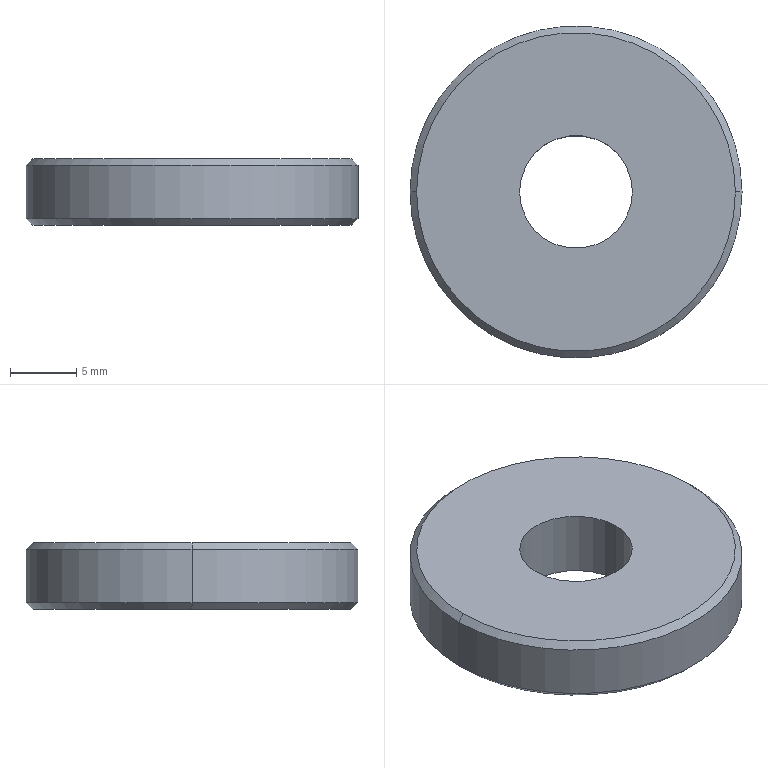Part | STEP file | PN_0013 Press plate | 1 solid | 10 faces | box 25 x 25 x 5 mm | volume 2151 mm3 | cylinder 4 | cone 4 | plane 2 | commonest cylinder face diameters 8.5 x2 25 x2
STEP:
#1=CARTESIAN_POINT('',(0.,0.,0.));
#2=DIRECTION('',(0.,0.,1.));
#3=DIRECTION('',(1.,0.,0.));
#4=AXIS2_PLACEMENT_3D('',#1,#2,#3);
#5=CARTESIAN_POINT('',(-4.25,0.,5.));
#6=VERTEX_POINT('',#5);
#7=CARTESIAN_POINT('',(-4.25,0.,0.));
#8=VERTEX_POINT('',#7);
#9=CARTESIAN_POINT('',(-4.25,0.,5.));
#10=DIRECTION('',(0.,0.,-1.));
#11=VECTOR('',#10,1.);
#12=LINE('',#9,#11);
#13=CARTESIAN_POINT('',(0.,0.,5.));
#14=DIRECTION('',(0.,0.,-1.));
#15=DIRECTION('',(-1.,0.,0.));
#16=AXIS2_PLACEMENT_3D('',#13,#14,#15);
#17=CYLINDRICAL_SURFACE('',#16,4.25);
#18=CARTESIAN_POINT('',(6.283,0.));
#19=DIRECTION('',(0.,1.));
#20=VECTOR('',#19,1.);
#21=LINE('',#18,#20);
#22=(GEOMETRIC_REPRESENTATION_CONTEXT(2)PARAMETRIC_REPRESENTATION_CONTEXT()REPRESENTATION_CONTEXT('',''));
#23=DEFINITIONAL_REPRESENTATION('',(#21),#22);
#24=PCURVE('',#17,#23);
#25=CARTESIAN_POINT('',(0.,0.,5.));
#26=DIRECTION('',(0.,0.,-1.));
#27=DIRECTION('',(-1.,0.,0.));
#28=AXIS2_PLACEMENT_3D('',#25,#26,#27);
#29=CYLINDRICAL_SURFACE('',#28,4.25);
#30=CARTESIAN_POINT('',(0.,0.));
#31=DIRECTION('',(0.,1.));
#32=VECTOR('',#31,1.);
#33=LINE('',#30,#32);
#34=(GEOMETRIC_REPRESENTATION_CONTEXT(2)PARAMETRIC_REPRESENTATION_CONTEXT()REPRESENTATION_CONTEXT('',''));
#35=DEFINITIONAL_REPRESENTATION('',(#33),#34);
#36=PCURVE('',#29,#35);
#37=SURFACE_CURVE('',#12,(#24,#36),.PCURVE_S1.);
#38=EDGE_CURVE('',#6,#8,#37,.T.);
#39=ORIENTED_EDGE('',*,*,#38,.T.);
#40=CARTESIAN_POINT('',(4.25,0.,0.));
#41=VERTEX_POINT('',#40);
#42=CARTESIAN_POINT('',(0.,0.,0.));
#43=DIRECTION('',(0.,0.,-1.));
#44=DIRECTION('',(-1.,0.,0.));
#45=AXIS2_PLACEMENT_3D('',#42,#43,#44);
#46=CIRCLE('',#45,4.25);
#47=CARTESIAN_POINT('',(0.,5.));
#48=DIRECTION('',(1.,0.));
#49=VECTOR('',#48,1.);
#50=LINE('',#47,#49);
#51=(GEOMETRIC_REPRESENTATION_CONTEXT(2)PARAMETRIC_REPRESENTATION_CONTEXT()REPRESENTATION_CONTEXT('',''));
#52=DEFINITIONAL_REPRESENTATION('',(#50),#51);
#53=PCURVE('',#17,#52);
#54=CARTESIAN_POINT('',(0.,0.,0.));
#55=DIRECTION('',(0.,0.,1.));
#56=DIRECTION('',(1.,0.,0.));
#57=AXIS2_PLACEMENT_3D('',#54,#55,#56);
#58=PLANE('',#57);
#59=CARTESIAN_POINT('',(-4.25,0.));
#60=CARTESIAN_POINT('',(-4.25,7.361));
#61=CARTESIAN_POINT('',(2.125,3.681));
#62=CARTESIAN_POINT('',(8.5,0.));
#63=CARTESIAN_POINT('',(2.125,-3.681));
#64=CARTESIAN_POINT('',(-4.25,-7.361));
#65=CARTESIAN_POINT('',(-4.25,0.));
#66=(BOUNDED_CURVE()B_SPLINE_CURVE(2,(#59,#60,#61,#62,#63,#64,#65),.UNSPECIFIED.,.T.,.F.)B_SPLINE_CURVE_WITH_KNOTS((1,2,2,2,2,1),(-2.094,0.,2.094,4.189,6.283,8.378),.UNSPECIFIED.)CURVE()GEOMETRIC_REPRESENTATION_ITEM()RATIONAL_B_SPLINE_CURVE((1.,0.5,1.,0.5,1.,0.5,1.))REPRESENTATION_ITEM(''));
#67=(GEOMETRIC_REPRESENTATION_CONTEXT(2)PARAMETRIC_REPRESENTATION_CONTEXT()REPRESENTATION_CONTEXT('',''));
#68=DEFINITIONAL_REPRESENTATION('',(#66),#67);
#69=PCURVE('',#58,#68);
#70=SURFACE_CURVE('',#46,(#53,#69),.PCURVE_S1.);
#71=EDGE_CURVE('',#41,#8,#70,.T.);
#72=ORIENTED_EDGE('',*,*,#71,.F.);
#73=CARTESIAN_POINT('',(4.25,0.,5.));
#74=VERTEX_POINT('',#73);
#75=CARTESIAN_POINT('',(4.25,0.,5.));
#76=DIRECTION('',(0.,0.,-1.));
#77=VECTOR('',#76,1.);
#78=LINE('',#75,#77);
#79=CARTESIAN_POINT('',(3.142,0.));
#80=DIRECTION('',(0.,1.));
#81=VECTOR('',#80,1.);
#82=LINE('',#79,#81);
#83=(GEOMETRIC_REPRESENTATION_CONTEXT(2)PARAMETRIC_REPRESENTATION_CONTEXT()REPRESENTATION_CONTEXT('',''));
#84=DEFINITIONAL_REPRESENTATION('',(#82),#83);
#85=PCURVE('',#17,#84);
#86=CARTESIAN_POINT('',(3.142,0.));
#87=DIRECTION('',(0.,1.));
#88=VECTOR('',#87,1.);
#89=LINE('',#86,#88);
#90=(GEOMETRIC_REPRESENTATION_CONTEXT(2)PARAMETRIC_REPRESENTATION_CONTEXT()REPRESENTATION_CONTEXT('',''));
#91=DEFINITIONAL_REPRESENTATION('',(#89),#90);
#92=PCURVE('',#29,#91);
#93=SURFACE_CURVE('',#78,(#85,#92),.PCURVE_S1.);
#94=EDGE_CURVE('',#74,#41,#93,.T.);
#95=ORIENTED_EDGE('',*,*,#94,.F.);
#96=CARTESIAN_POINT('',(0.,0.,5.));
#97=DIRECTION('',(0.,0.,-1.));
#98=DIRECTION('',(-1.,0.,0.));
#99=AXIS2_PLACEMENT_3D('',#96,#97,#98);
#100=CIRCLE('',#99,4.25);
#101=CARTESIAN_POINT('',(0.,0.));
#102=DIRECTION('',(1.,0.));
#103=VECTOR('',#102,1.);
#104=LINE('',#101,#103);
#105=(GEOMETRIC_REPRESENTATION_CONTEXT(2)PARAMETRIC_REPRESENTATION_CONTEXT()REPRESENTATION_CONTEXT('',''));
#106=DEFINITIONAL_REPRESENTATION('',(#104),#105);
#107=PCURVE('',#17,#106);
#108=CARTESIAN_POINT('',(0.,0.,5.));
#109=DIRECTION('',(0.,0.,1.));
#110=DIRECTION('',(1.,0.,0.));
#111=AXIS2_PLACEMENT_3D('',#108,#109,#110);
#112=PLANE('',#111);
#113=CARTESIAN_POINT('',(-4.25,0.));
#114=CARTESIAN_POINT('',(-4.25,7.361));
#115=CARTESIAN_POINT('',(2.125,3.681));
#116=CARTESIAN_POINT('',(8.5,0.));
#117=CARTESIAN_POINT('',(2.125,-3.681));
#118=CARTESIAN_POINT('',(-4.25,-7.361));
#119=CARTESIAN_POINT('',(-4.25,0.));
#120=(BOUNDED_CURVE()B_SPLINE_CURVE(2,(#113,#114,#115,#116,#117,#118,#119),.UNSPECIFIED.,.T.,.F.)B_SPLINE_CURVE_WITH_KNOTS((1,2,2,2,2,1),(-2.094,0.,2.094,4.189,6.283,8.378),.UNSPECIFIED.)CURVE()GEOMETRIC_REPRESENTATION_ITEM()RATIONAL_B_SPLINE_CURVE((1.,0.5,1.,0.5,1.,0.5,1.))REPRESENTATION_ITEM(''));
#121=(GEOMETRIC_REPRESENTATION_CONTEXT(2)PARAMETRIC_REPRESENTATION_CONTEXT()REPRESENTATION_CONTEXT('',''));
#122=DEFINITIONAL_REPRESENTATION('',(#120),#121);
#123=PCURVE('',#112,#122);
#124=SURFACE_CURVE('',#100,(#107,#123),.PCURVE_S1.);
#125=EDGE_CURVE('',#74,#6,#124,.T.);
#126=ORIENTED_EDGE('',*,*,#125,.T.);
#127=EDGE_LOOP('',(#39,#72,#95,#126));
#128=FACE_BOUND('',#127,.F.);
#129=ADVANCED_FACE('',(#128),#17,.F.);
#130=CARTESIAN_POINT('',(12.,0.,0.));
#131=VERTEX_POINT('',#130);
#132=CARTESIAN_POINT('',(-12.,0.,0.));
#133=VERTEX_POINT('',#132);
#134=CARTESIAN_POINT('',(0.,0.,0.));
#135=DIRECTION('',(0.,0.,1.));
#136=DIRECTION('',(1.,0.,0.));
#137=AXIS2_PLACEMENT_3D('',#134,#135,#136);
#138=CIRCLE('',#137,12.);
#139=CARTESIAN_POINT('',(0.,0.,0.5));
#140=DIRECTION('',(0.,0.,1.));
#141=DIRECTION('',(1.,0.,0.));
#142=AXIS2_PLACEMENT_3D('',#139,#140,#141);
#143=CONICAL_SURFACE('',#142,12.5,0.7854);
#144=CARTESIAN_POINT('',(0.,-0.5));
#145=DIRECTION('',(1.,0.));
#146=VECTOR('',#145,1.);
#147=LINE('',#144,#146);
#148=(GEOMETRIC_REPRESENTATION_CONTEXT(2)PARAMETRIC_REPRESENTATION_CONTEXT()REPRESENTATION_CONTEXT('',''));
#149=DEFINITIONAL_REPRESENTATION('',(#147),#148);
#150=PCURVE('',#143,#149);
#151=CARTESIAN_POINT('',(0.,0.));
#152=DIRECTION('',(1.,0.));
#153=AXIS2_PLACEMENT_2D('',#151,#152);
#154=CIRCLE('',#153,12.);
#155=(GEOMETRIC_REPRESENTATION_CONTEXT(2)PARAMETRIC_REPRESENTATION_CONTEXT()REPRESENTATION_CONTEXT('',''));
#156=DEFINITIONAL_REPRESENTATION('',(#154),#155);
#157=PCURVE('',#58,#156);
#158=SURFACE_CURVE('',#138,(#150,#157),.PCURVE_S1.);
#159=EDGE_CURVE('',#131,#133,#158,.T.);
#160=ORIENTED_EDGE('',*,*,#159,.T.);
#161=CARTESIAN_POINT('',(-12.5,0.,0.5));
#162=VERTEX_POINT('',#161);
#163=CARTESIAN_POINT('',(-12.5,0.,0.5));
#164=DIRECTION('',(-0.7071,0.,0.7071));
#165=VECTOR('',#164,1.);
#166=LINE('',#163,#165);
#167=CARTESIAN_POINT('',(3.142,0.));
#168=DIRECTION('',(0.,1.));
#169=VECTOR('',#168,1.);
#170=LINE('',#167,#169);
#171=(GEOMETRIC_REPRESENTATION_CONTEXT(2)PARAMETRIC_REPRESENTATION_CONTEXT()REPRESENTATION_CONTEXT('',''));
#172=DEFINITIONAL_REPRESENTATION('',(#170),#171);
#173=PCURVE('',#143,#172);
#174=CARTESIAN_POINT('',(0.,0.,0.5));
#175=DIRECTION('',(0.,0.,1.));
#176=DIRECTION('',(1.,0.,0.));
#177=AXIS2_PLACEMENT_3D('',#174,#175,#176);
#178=CONICAL_SURFACE('',#177,12.5,0.7854);
#179=CARTESIAN_POINT('',(3.142,0.));
#180=DIRECTION('',(0.,1.));
#181=VECTOR('',#180,1.);
#182=LINE('',#179,#181);
#183=(GEOMETRIC_REPRESENTATION_CONTEXT(2)PARAMETRIC_REPRESENTATION_CONTEXT()REPRESENTATION_CONTEXT('',''));
#184=DEFINITIONAL_REPRESENTATION('',(#182),#183);
#185=PCURVE('',#178,#184);
#186=SURFACE_CURVE('',#166,(#173,#185),.PCURVE_S1.);
#187=EDGE_CURVE('',#133,#162,#186,.T.);
#188=ORIENTED_EDGE('',*,*,#187,.T.);
#189=CARTESIAN_POINT('',(12.5,0.,0.5));
#190=VERTEX_POINT('',#189);
#191=CARTESIAN_POINT('',(0.,0.,0.5));
#192=DIRECTION('',(0.,0.,-1.));
#193=DIRECTION('',(1.,0.,0.));
#194=AXIS2_PLACEMENT_3D('',#191,#192,#193);
#195=CIRCLE('',#194,12.5);
#196=CARTESIAN_POINT('',(6.283,0.));
#197=DIRECTION('',(-1.,0.));
#198=VECTOR('',#197,1.);
#199=LINE('',#196,#198);
#200=(GEOMETRIC_REPRESENTATION_CONTEXT(2)PARAMETRIC_REPRESENTATION_CONTEXT()REPRESENTATION_CONTEXT('',''));
#201=DEFINITIONAL_REPRESENTATION('',(#199),#200);
#202=PCURVE('',#143,#201);
#203=CARTESIAN_POINT('',(0.,0.,5.));
#204=DIRECTION('',(0.,0.,-1.));
#205=DIRECTION('',(-1.,0.,0.));
#206=AXIS2_PLACEMENT_3D('',#203,#204,#205);
#207=CYLINDRICAL_SURFACE('',#206,12.5);
#208=CARTESIAN_POINT('',(-3.142,4.5));
#209=DIRECTION('',(1.,0.));
#210=VECTOR('',#209,1.);
#211=LINE('',#208,#210);
#212=(GEOMETRIC_REPRESENTATION_CONTEXT(2)PARAMETRIC_REPRESENTATION_CONTEXT()REPRESENTATION_CONTEXT('',''));
#213=DEFINITIONAL_REPRESENTATION('',(#211),#212);
#214=PCURVE('',#207,#213);
#215=SURFACE_CURVE('',#195,(#202,#214),.PCURVE_S1.);
#216=EDGE_CURVE('',#162,#190,#215,.T.);
#217=ORIENTED_EDGE('',*,*,#216,.T.);
#218=CARTESIAN_POINT('',(12.5,0.,0.5));
#219=DIRECTION('',(0.7071,0.,0.7071));
#220=VECTOR('',#219,1.);
#221=LINE('',#218,#220);
#222=CARTESIAN_POINT('',(0.,0.));
#223=DIRECTION('',(0.,1.));
#224=VECTOR('',#223,1.);
#225=LINE('',#222,#224);
#226=(GEOMETRIC_REPRESENTATION_CONTEXT(2)PARAMETRIC_REPRESENTATION_CONTEXT()REPRESENTATION_CONTEXT('',''));
#227=DEFINITIONAL_REPRESENTATION('',(#225),#226);
#228=PCURVE('',#143,#227);
#229=CARTESIAN_POINT('',(6.283,0.));
#230=DIRECTION('',(0.,1.));
#231=VECTOR('',#230,1.);
#232=LINE('',#229,#231);
#233=(GEOMETRIC_REPRESENTATION_CONTEXT(2)PARAMETRIC_REPRESENTATION_CONTEXT()REPRESENTATION_CONTEXT('',''));
#234=DEFINITIONAL_REPRESENTATION('',(#232),#233);
#235=PCURVE('',#178,#234);
#236=SURFACE_CURVE('',#221,(#228,#235),.PCURVE_S1.);
#237=EDGE_CURVE('',#131,#190,#236,.T.);
#238=ORIENTED_EDGE('',*,*,#237,.F.);
#239=EDGE_LOOP('',(#160,#188,#217,#238));
#240=FACE_BOUND('',#239,.T.);
#241=ADVANCED_FACE('',(#240),#143,.T.);
#242=CARTESIAN_POINT('',(-12.5,0.,4.5));
#243=VERTEX_POINT('',#242);
#244=CARTESIAN_POINT('',(12.5,0.,4.5));
#245=VERTEX_POINT('',#244);
#246=CARTESIAN_POINT('',(0.,0.,4.5));
#247=DIRECTION('',(0.,0.,-1.));
#248=DIRECTION('',(-1.,0.,0.));
#249=AXIS2_PLACEMENT_3D('',#246,#247,#248);
#250=CIRCLE('',#249,12.5);
#251=CARTESIAN_POINT('',(0.,0.5));
#252=DIRECTION('',(1.,0.));
#253=VECTOR('',#252,1.);
#254=LINE('',#251,#253);
#255=(GEOMETRIC_REPRESENTATION_CONTEXT(2)PARAMETRIC_REPRESENTATION_CONTEXT()REPRESENTATION_CONTEXT('',''));
#256=DEFINITIONAL_REPRESENTATION('',(#254),#255);
#257=PCURVE('',#207,#256);
#258=CARTESIAN_POINT('',(0.,0.,4.5));
#259=DIRECTION('',(0.,0.,-1.));
#260=DIRECTION('',(-1.,0.,0.));
#261=AXIS2_PLACEMENT_3D('',#258,#259,#260);
#262=CONICAL_SURFACE('',#261,12.5,0.7854);
#263=CARTESIAN_POINT('',(0.,0.));
#264=DIRECTION('',(1.,0.));
#265=VECTOR('',#264,1.);
#266=LINE('',#263,#265);
#267=(GEOMETRIC_REPRESENTATION_CONTEXT(2)PARAMETRIC_REPRESENTATION_CONTEXT()REPRESENTATION_CONTEXT('',''));
#268=DEFINITIONAL_REPRESENTATION('',(#266),#267);
#269=PCURVE('',#262,#268);
#270=SURFACE_CURVE('',#250,(#257,#269),.PCURVE_S1.);
#271=EDGE_CURVE('',#243,#245,#270,.T.);
#272=ORIENTED_EDGE('',*,*,#271,.T.);
#273=CARTESIAN_POINT('',(12.5,0.,5.));
#274=DIRECTION('',(0.,0.,-1.));
#275=VECTOR('',#274,1.);
#276=LINE('',#273,#275);
#277=CARTESIAN_POINT('',(3.142,0.));
#278=DIRECTION('',(0.,1.));
#279=VECTOR('',#278,1.);
#280=LINE('',#277,#279);
#281=(GEOMETRIC_REPRESENTATION_CONTEXT(2)PARAMETRIC_REPRESENTATION_CONTEXT()REPRESENTATION_CONTEXT('',''));
#282=DEFINITIONAL_REPRESENTATION('',(#280),#281);
#283=PCURVE('',#207,#282);
#284=CARTESIAN_POINT('',(0.,0.,5.));
#285=DIRECTION('',(0.,0.,-1.));
#286=DIRECTION('',(-1.,0.,0.));
#287=AXIS2_PLACEMENT_3D('',#284,#285,#286);
#288=CYLINDRICAL_SURFACE('',#287,12.5);
#289=CARTESIAN_POINT('',(3.142,0.));
#290=DIRECTION('',(0.,1.));
#291=VECTOR('',#290,1.);
#292=LINE('',#289,#291);
#293=(GEOMETRIC_REPRESENTATION_CONTEXT(2)PARAMETRIC_REPRESENTATION_CONTEXT()REPRESENTATION_CONTEXT('',''));
#294=DEFINITIONAL_REPRESENTATION('',(#292),#293);
#295=PCURVE('',#288,#294);
#296=SURFACE_CURVE('',#276,(#283,#295),.PCURVE_S1.);
#297=EDGE_CURVE('',#245,#190,#296,.T.);
#298=ORIENTED_EDGE('',*,*,#297,.T.);
#299=ORIENTED_EDGE('',*,*,#216,.F.);
#300=CARTESIAN_POINT('',(-12.5,0.,5.));
#301=DIRECTION('',(0.,0.,-1.));
#302=VECTOR('',#301,1.);
#303=LINE('',#300,#302);
#304=CARTESIAN_POINT('',(0.,0.));
#305=DIRECTION('',(0.,1.));
#306=VECTOR('',#305,1.);
#307=LINE('',#304,#306);
#308=(GEOMETRIC_REPRESENTATION_CONTEXT(2)PARAMETRIC_REPRESENTATION_CONTEXT()REPRESENTATION_CONTEXT('',''));
#309=DEFINITIONAL_REPRESENTATION('',(#307),#308);
#310=PCURVE('',#207,#309);
#311=CARTESIAN_POINT('',(6.283,0.));
#312=DIRECTION('',(0.,1.));
#313=VECTOR('',#312,1.);
#314=LINE('',#311,#313);
#315=(GEOMETRIC_REPRESENTATION_CONTEXT(2)PARAMETRIC_REPRESENTATION_CONTEXT()REPRESENTATION_CONTEXT('',''));
#316=DEFINITIONAL_REPRESENTATION('',(#314),#315);
#317=PCURVE('',#288,#316);
#318=SURFACE_CURVE('',#303,(#310,#317),.PCURVE_S1.);
#319=EDGE_CURVE('',#243,#162,#318,.T.);
#320=ORIENTED_EDGE('',*,*,#319,.F.);
#321=EDGE_LOOP('',(#272,#298,#299,#320));
#322=FACE_BOUND('',#321,.T.);
#323=ADVANCED_FACE('',(#322),#207,.T.);
#324=CARTESIAN_POINT('',(12.,0.,5.));
#325=VERTEX_POINT('',#324);
#326=CARTESIAN_POINT('',(-12.,0.,5.));
#327=VERTEX_POINT('',#326);
#328=CARTESIAN_POINT('',(0.,0.,5.));
#329=DIRECTION('',(0.,0.,1.));
#330=DIRECTION('',(-1.,0.,0.));
#331=AXIS2_PLACEMENT_3D('',#328,#329,#330);
#332=CIRCLE('',#331,12.);
#333=CARTESIAN_POINT('',(6.283,-0.5));
#334=DIRECTION('',(-1.,0.));
#335=VECTOR('',#334,1.);
#336=LINE('',#333,#335);
#337=(GEOMETRIC_REPRESENTATION_CONTEXT(2)PARAMETRIC_REPRESENTATION_CONTEXT()REPRESENTATION_CONTEXT('',''));
#338=DEFINITIONAL_REPRESENTATION('',(#336),#337);
#339=PCURVE('',#262,#338);
#340=CARTESIAN_POINT('',(0.,0.));
#341=DIRECTION('',(-1.,0.));
#342=AXIS2_PLACEMENT_2D('',#340,#341);
#343=CIRCLE('',#342,12.);
#344=(GEOMETRIC_REPRESENTATION_CONTEXT(2)PARAMETRIC_REPRESENTATION_CONTEXT()REPRESENTATION_CONTEXT('',''));
#345=DEFINITIONAL_REPRESENTATION('',(#343),#344);
#346=PCURVE('',#112,#345);
#347=SURFACE_CURVE('',#332,(#339,#346),.PCURVE_S1.);
#348=EDGE_CURVE('',#325,#327,#347,.T.);
#349=ORIENTED_EDGE('',*,*,#348,.F.);
#350=CARTESIAN_POINT('',(12.5,0.,4.5));
#351=DIRECTION('',(0.7071,0.,-0.7071));
#352=VECTOR('',#351,1.);
#353=LINE('',#350,#352);
#354=CARTESIAN_POINT('',(3.142,0.));
#355=DIRECTION('',(0.,1.));
#356=VECTOR('',#355,1.);
#357=LINE('',#354,#356);
#358=(GEOMETRIC_REPRESENTATION_CONTEXT(2)PARAMETRIC_REPRESENTATION_CONTEXT()REPRESENTATION_CONTEXT('',''));
#359=DEFINITIONAL_REPRESENTATION('',(#357),#358);
#360=PCURVE('',#262,#359);
#361=CARTESIAN_POINT('',(0.,0.,4.5));
#362=DIRECTION('',(0.,0.,-1.));
#363=DIRECTION('',(-1.,0.,0.));
#364=AXIS2_PLACEMENT_3D('',#361,#362,#363);
#365=CONICAL_SURFACE('',#364,12.5,0.7854);
#366=CARTESIAN_POINT('',(3.142,0.));
#367=DIRECTION('',(0.,1.));
#368=VECTOR('',#367,1.);
#369=LINE('',#366,#368);
#370=(GEOMETRIC_REPRESENTATION_CONTEXT(2)PARAMETRIC_REPRESENTATION_CONTEXT()REPRESENTATION_CONTEXT('',''));
#371=DEFINITIONAL_REPRESENTATION('',(#369),#370);
#372=PCURVE('',#365,#371);
#373=SURFACE_CURVE('',#353,(#360,#372),.PCURVE_S1.);
#374=EDGE_CURVE('',#325,#245,#373,.T.);
#375=ORIENTED_EDGE('',*,*,#374,.T.);
#376=ORIENTED_EDGE('',*,*,#271,.F.);
#377=CARTESIAN_POINT('',(-12.5,0.,4.5));
#378=DIRECTION('',(-0.7071,0.,-0.7071));
#379=VECTOR('',#378,1.);
#380=LINE('',#377,#379);
#381=CARTESIAN_POINT('',(0.,0.));
#382=DIRECTION('',(0.,1.));
#383=VECTOR('',#382,1.);
#384=LINE('',#381,#383);
#385=(GEOMETRIC_REPRESENTATION_CONTEXT(2)PARAMETRIC_REPRESENTATION_CONTEXT()REPRESENTATION_CONTEXT('',''));
#386=DEFINITIONAL_REPRESENTATION('',(#384),#385);
#387=PCURVE('',#262,#386);
#388=CARTESIAN_POINT('',(6.283,0.));
#389=DIRECTION('',(0.,1.));
#390=VECTOR('',#389,1.);
#391=LINE('',#388,#390);
#392=(GEOMETRIC_REPRESENTATION_CONTEXT(2)PARAMETRIC_REPRESENTATION_CONTEXT()REPRESENTATION_CONTEXT('',''));
#393=DEFINITIONAL_REPRESENTATION('',(#391),#392);
#394=PCURVE('',#365,#393);
#395=SURFACE_CURVE('',#380,(#387,#394),.PCURVE_S1.);
#396=EDGE_CURVE('',#327,#243,#395,.T.);
#397=ORIENTED_EDGE('',*,*,#396,.F.);
#398=EDGE_LOOP('',(#349,#375,#376,#397));
#399=FACE_BOUND('',#398,.T.);
#400=ADVANCED_FACE('',(#399),#262,.T.);
#401=CARTESIAN_POINT('',(0.,0.,0.));
#402=DIRECTION('',(0.,0.,-1.));
#403=DIRECTION('',(-1.,0.,0.));
#404=AXIS2_PLACEMENT_3D('',#401,#402,#403);
#405=CIRCLE('',#404,4.25);
#406=CARTESIAN_POINT('',(-4.25,0.));
#407=CARTESIAN_POINT('',(-4.25,7.361));
#408=CARTESIAN_POINT('',(2.125,3.681));
#409=CARTESIAN_POINT('',(8.5,0.));
#410=CARTESIAN_POINT('',(2.125,-3.681));
#411=CARTESIAN_POINT('',(-4.25,-7.361));
#412=CARTESIAN_POINT('',(-4.25,0.));
#413=(BOUNDED_CURVE()B_SPLINE_CURVE(2,(#406,#407,#408,#409,#410,#411,#412),.UNSPECIFIED.,.T.,.F.)B_SPLINE_CURVE_WITH_KNOTS((1,2,2,2,2,1),(-2.094,0.,2.094,4.189,6.283,8.378),.UNSPECIFIED.)CURVE()GEOMETRIC_REPRESENTATION_ITEM()RATIONAL_B_SPLINE_CURVE((1.,0.5,1.,0.5,1.,0.5,1.))REPRESENTATION_ITEM(''));
#414=(GEOMETRIC_REPRESENTATION_CONTEXT(2)PARAMETRIC_REPRESENTATION_CONTEXT()REPRESENTATION_CONTEXT('',''));
#415=DEFINITIONAL_REPRESENTATION('',(#413),#414);
#416=PCURVE('',#58,#415);
#417=CARTESIAN_POINT('',(0.,5.));
#418=DIRECTION('',(1.,0.));
#419=VECTOR('',#418,1.);
#420=LINE('',#417,#419);
#421=(GEOMETRIC_REPRESENTATION_CONTEXT(2)PARAMETRIC_REPRESENTATION_CONTEXT()REPRESENTATION_CONTEXT('',''));
#422=DEFINITIONAL_REPRESENTATION('',(#420),#421);
#423=PCURVE('',#29,#422);
#424=SURFACE_CURVE('',#405,(#416,#423),.PCURVE_S1.);
#425=EDGE_CURVE('',#8,#41,#424,.T.);
#426=ORIENTED_EDGE('',*,*,#425,.F.);
#427=ORIENTED_EDGE('',*,*,#71,.F.);
#428=EDGE_LOOP('',(#426,#427));
#429=FACE_BOUND('',#428,.T.);
#430=ORIENTED_EDGE('',*,*,#159,.F.);
#431=CARTESIAN_POINT('',(0.,0.,0.));
#432=DIRECTION('',(0.,0.,1.));
#433=DIRECTION('',(1.,0.,0.));
#434=AXIS2_PLACEMENT_3D('',#431,#432,#433);
#435=CIRCLE('',#434,12.);
#436=CARTESIAN_POINT('',(0.,0.));
#437=DIRECTION('',(1.,0.));
#438=AXIS2_PLACEMENT_2D('',#436,#437);
#439=CIRCLE('',#438,12.);
#440=(GEOMETRIC_REPRESENTATION_CONTEXT(2)PARAMETRIC_REPRESENTATION_CONTEXT()REPRESENTATION_CONTEXT('',''));
#441=DEFINITIONAL_REPRESENTATION('',(#439),#440);
#442=PCURVE('',#58,#441);
#443=CARTESIAN_POINT('',(0.,-0.5));
#444=DIRECTION('',(1.,0.));
#445=VECTOR('',#444,1.);
#446=LINE('',#443,#445);
#447=(GEOMETRIC_REPRESENTATION_CONTEXT(2)PARAMETRIC_REPRESENTATION_CONTEXT()REPRESENTATION_CONTEXT('',''));
#448=DEFINITIONAL_REPRESENTATION('',(#446),#447);
#449=PCURVE('',#178,#448);
#450=SURFACE_CURVE('',#435,(#442,#449),.PCURVE_S1.);
#451=EDGE_CURVE('',#133,#131,#450,.T.);
#452=ORIENTED_EDGE('',*,*,#451,.F.);
#453=EDGE_LOOP('',(#430,#452));
#454=FACE_BOUND('',#453,.T.);
#455=ADVANCED_FACE('',(#429,#454),#58,.F.);
#456=ORIENTED_EDGE('',*,*,#425,.F.);
#457=ORIENTED_EDGE('',*,*,#38,.F.);
#458=CARTESIAN_POINT('',(0.,0.,5.));
#459=DIRECTION('',(0.,0.,-1.));
#460=DIRECTION('',(-1.,0.,0.));
#461=AXIS2_PLACEMENT_3D('',#458,#459,#460);
#462=CIRCLE('',#461,4.25);
#463=CARTESIAN_POINT('',(0.,0.));
#464=DIRECTION('',(1.,0.));
#465=VECTOR('',#464,1.);
#466=LINE('',#463,#465);
#467=(GEOMETRIC_REPRESENTATION_CONTEXT(2)PARAMETRIC_REPRESENTATION_CONTEXT()REPRESENTATION_CONTEXT('',''));
#468=DEFINITIONAL_REPRESENTATION('',(#466),#467);
#469=PCURVE('',#29,#468);
#470=CARTESIAN_POINT('',(-4.25,0.));
#471=CARTESIAN_POINT('',(-4.25,7.361));
#472=CARTESIAN_POINT('',(2.125,3.681));
#473=CARTESIAN_POINT('',(8.5,0.));
#474=CARTESIAN_POINT('',(2.125,-3.681));
#475=CARTESIAN_POINT('',(-4.25,-7.361));
#476=CARTESIAN_POINT('',(-4.25,0.));
#477=(BOUNDED_CURVE()B_SPLINE_CURVE(2,(#470,#471,#472,#473,#474,#475,#476),.UNSPECIFIED.,.T.,.F.)B_SPLINE_CURVE_WITH_KNOTS((1,2,2,2,2,1),(-2.094,0.,2.094,4.189,6.283,8.378),.UNSPECIFIED.)CURVE()GEOMETRIC_REPRESENTATION_ITEM()RATIONAL_B_SPLINE_CURVE((1.,0.5,1.,0.5,1.,0.5,1.))REPRESENTATION_ITEM(''));
#478=(GEOMETRIC_REPRESENTATION_CONTEXT(2)PARAMETRIC_REPRESENTATION_CONTEXT()REPRESENTATION_CONTEXT('',''));
#479=DEFINITIONAL_REPRESENTATION('',(#477),#478);
#480=PCURVE('',#112,#479);
#481=SURFACE_CURVE('',#462,(#469,#480),.PCURVE_S1.);
#482=EDGE_CURVE('',#6,#74,#481,.T.);
#483=ORIENTED_EDGE('',*,*,#482,.T.);
#484=ORIENTED_EDGE('',*,*,#94,.T.);
#485=EDGE_LOOP('',(#456,#457,#483,#484));
#486=FACE_BOUND('',#485,.F.);
#487=ADVANCED_FACE('',(#486),#29,.F.);
#488=ORIENTED_EDGE('',*,*,#187,.F.);
#489=ORIENTED_EDGE('',*,*,#451,.T.);
#490=ORIENTED_EDGE('',*,*,#237,.T.);
#491=CARTESIAN_POINT('',(0.,0.,0.5));
#492=DIRECTION('',(0.,0.,-1.));
#493=DIRECTION('',(1.,0.,0.));
#494=AXIS2_PLACEMENT_3D('',#491,#492,#493);
#495=CIRCLE('',#494,12.5);
#496=CARTESIAN_POINT('',(6.283,0.));
#497=DIRECTION('',(-1.,0.));
#498=VECTOR('',#497,1.);
#499=LINE('',#496,#498);
#500=(GEOMETRIC_REPRESENTATION_CONTEXT(2)PARAMETRIC_REPRESENTATION_CONTEXT()REPRESENTATION_CONTEXT('',''));
#501=DEFINITIONAL_REPRESENTATION('',(#499),#500);
#502=PCURVE('',#178,#501);
#503=CARTESIAN_POINT('',(3.142,4.5));
#504=DIRECTION('',(1.,0.));
#505=VECTOR('',#504,1.);
#506=LINE('',#503,#505);
#507=(GEOMETRIC_REPRESENTATION_CONTEXT(2)PARAMETRIC_REPRESENTATION_CONTEXT()REPRESENTATION_CONTEXT('',''));
#508=DEFINITIONAL_REPRESENTATION('',(#506),#507);
#509=PCURVE('',#288,#508);
#510=SURFACE_CURVE('',#495,(#502,#509),.PCURVE_S1.);
#511=EDGE_CURVE('',#190,#162,#510,.T.);
#512=ORIENTED_EDGE('',*,*,#511,.T.);
#513=EDGE_LOOP('',(#488,#489,#490,#512));
#514=FACE_BOUND('',#513,.T.);
#515=ADVANCED_FACE('',(#514),#178,.T.);
#516=ORIENTED_EDGE('',*,*,#482,.T.);
#517=ORIENTED_EDGE('',*,*,#125,.T.);
#518=EDGE_LOOP('',(#516,#517));
#519=FACE_BOUND('',#518,.T.);
#520=CARTESIAN_POINT('',(0.,0.,5.));
#521=DIRECTION('',(0.,0.,1.));
#522=DIRECTION('',(-1.,0.,0.));
#523=AXIS2_PLACEMENT_3D('',#520,#521,#522);
#524=CIRCLE('',#523,12.);
#525=CARTESIAN_POINT('',(0.,0.));
#526=DIRECTION('',(-1.,0.));
#527=AXIS2_PLACEMENT_2D('',#525,#526);
#528=CIRCLE('',#527,12.);
#529=(GEOMETRIC_REPRESENTATION_CONTEXT(2)PARAMETRIC_REPRESENTATION_CONTEXT()REPRESENTATION_CONTEXT('',''));
#530=DEFINITIONAL_REPRESENTATION('',(#528),#529);
#531=PCURVE('',#112,#530);
#532=CARTESIAN_POINT('',(6.283,-0.5));
#533=DIRECTION('',(-1.,0.));
#534=VECTOR('',#533,1.);
#535=LINE('',#532,#534);
#536=(GEOMETRIC_REPRESENTATION_CONTEXT(2)PARAMETRIC_REPRESENTATION_CONTEXT()REPRESENTATION_CONTEXT('',''));
#537=DEFINITIONAL_REPRESENTATION('',(#535),#536);
#538=PCURVE('',#365,#537);
#539=SURFACE_CURVE('',#524,(#531,#538),.PCURVE_S1.);
#540=EDGE_CURVE('',#327,#325,#539,.T.);
#541=ORIENTED_EDGE('',*,*,#540,.T.);
#542=ORIENTED_EDGE('',*,*,#348,.T.);
#543=EDGE_LOOP('',(#541,#542));
#544=FACE_BOUND('',#543,.T.);
#545=ADVANCED_FACE('',(#519,#544),#112,.T.);
#546=ORIENTED_EDGE('',*,*,#297,.F.);
#547=CARTESIAN_POINT('',(0.,0.,4.5));
#548=DIRECTION('',(0.,0.,-1.));
#549=DIRECTION('',(-1.,0.,0.));
#550=AXIS2_PLACEMENT_3D('',#547,#548,#549);
#551=CIRCLE('',#550,12.5);
#552=CARTESIAN_POINT('',(0.,0.5));
#553=DIRECTION('',(1.,0.));
#554=VECTOR('',#553,1.);
#555=LINE('',#552,#554);
#556=(GEOMETRIC_REPRESENTATION_CONTEXT(2)PARAMETRIC_REPRESENTATION_CONTEXT()REPRESENTATION_CONTEXT('',''));
#557=DEFINITIONAL_REPRESENTATION('',(#555),#556);
#558=PCURVE('',#288,#557);
#559=CARTESIAN_POINT('',(0.,0.));
#560=DIRECTION('',(1.,0.));
#561=VECTOR('',#560,1.);
#562=LINE('',#559,#561);
#563=(GEOMETRIC_REPRESENTATION_CONTEXT(2)PARAMETRIC_REPRESENTATION_CONTEXT()REPRESENTATION_CONTEXT('',''));
#564=DEFINITIONAL_REPRESENTATION('',(#562),#563);
#565=PCURVE('',#365,#564);
#566=SURFACE_CURVE('',#551,(#558,#565),.PCURVE_S1.);
#567=EDGE_CURVE('',#245,#243,#566,.T.);
#568=ORIENTED_EDGE('',*,*,#567,.T.);
#569=ORIENTED_EDGE('',*,*,#319,.T.);
#570=ORIENTED_EDGE('',*,*,#511,.F.);
#571=EDGE_LOOP('',(#546,#568,#569,#570));
#572=FACE_BOUND('',#571,.T.);
#573=ADVANCED_FACE('',(#572),#288,.T.);
#574=ORIENTED_EDGE('',*,*,#374,.F.);
#575=ORIENTED_EDGE('',*,*,#540,.F.);
#576=ORIENTED_EDGE('',*,*,#396,.T.);
#577=ORIENTED_EDGE('',*,*,#567,.F.);
#578=EDGE_LOOP('',(#574,#575,#576,#577));
#579=FACE_BOUND('',#578,.T.);
#580=ADVANCED_FACE('',(#579),#365,.T.);
#581=CLOSED_SHELL('',(#129,#241,#323,#400,#455,#487,#515,#545,#573,#580));
#582=MANIFOLD_SOLID_BREP('',#581);
#583=(LENGTH_UNIT()NAMED_UNIT(*)SI_UNIT(.MILLI.,.METRE.));
#584=UNCERTAINTY_MEASURE_WITH_UNIT(LENGTH_MEASURE(0.0000001),#583,'','');
#585=(NAMED_UNIT(*)PLANE_ANGLE_UNIT()SI_UNIT($,.RADIAN.));
#586=(NAMED_UNIT(*)SI_UNIT($,.STERADIAN.)SOLID_ANGLE_UNIT());
#587=(GEOMETRIC_REPRESENTATION_CONTEXT(3)GLOBAL_UNCERTAINTY_ASSIGNED_CONTEXT((#584))GLOBAL_UNIT_ASSIGNED_CONTEXT((#583,#585,#586))REPRESENTATION_CONTEXT('',''));
#588=ADVANCED_BREP_SHAPE_REPRESENTATION('',(#4,#582),#587);